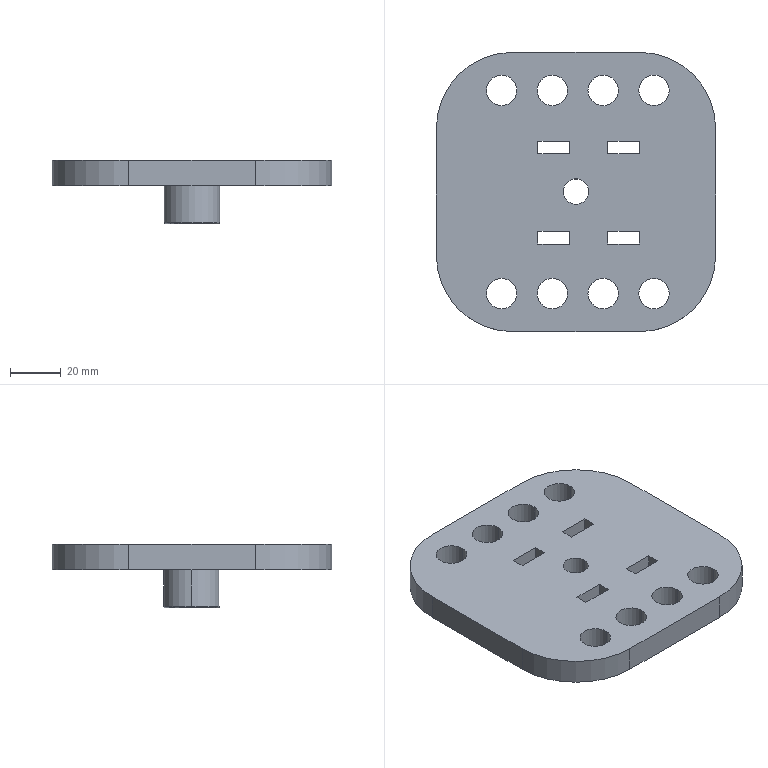Part | SolidWorks | features Fillet 2, ICE 2, Extrusion 1 | 1 solid | 51 faces | box 110 x 110 x 25 mm | volume 105460 mm3 | cylinder 24 | plane 23 | torus 4 | commonest cylinder face diameters 12 x16 60 x4 10 x2 22 x2